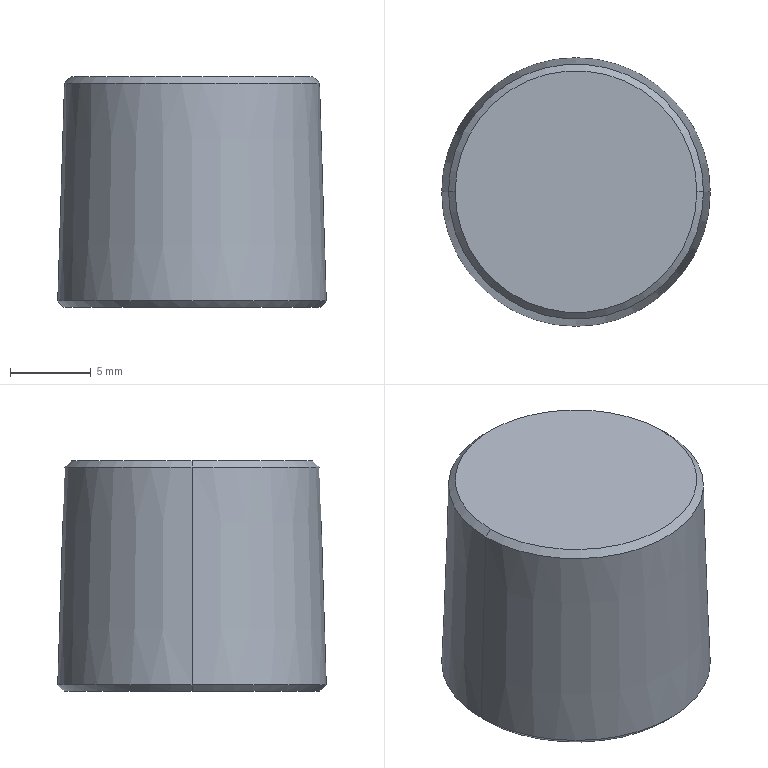Part | Creo | 1 solid | 15 faces | box 16.637 x 16.637 x 14.3 mm | volume 2739 mm3 | plane 9 | cone 6
STEP:
#1=CARTESIAN_POINT('',(-31.754,182.,-30.7));
#2=VERTEX_POINT('',#1);
#3=CARTESIAN_POINT('',(-46.729,182.,-30.7));
#4=VERTEX_POINT('',#3);
#5=CARTESIAN_POINT('',(-39.242,182.,-30.7));
#6=DIRECTION('',(0.,0.,1.));
#7=DIRECTION('',(1.,0.,0.));
#8=AXIS2_PLACEMENT_3D('',#5,#6,#7);
#9=CIRCLE('',#8,7.488);
#10=EDGE_CURVE('',#2,#4,#9,.T.);
#11=ORIENTED_EDGE('',*,*,#10,.F.);
#12=CARTESIAN_POINT('',(-39.242,182.,-30.7));
#13=DIRECTION('',(0.,0.,1.));
#14=DIRECTION('',(-1.,0.,0.));
#15=AXIS2_PLACEMENT_3D('',#12,#13,#14);
#16=CIRCLE('',#15,7.488);
#17=EDGE_CURVE('',#4,#2,#16,.T.);
#18=ORIENTED_EDGE('',*,*,#17,.F.);
#19=EDGE_LOOP('',(#11,#18));
#20=FACE_OUTER_BOUND('',#19,.F.);
#21=CARTESIAN_POINT('',(-47.129,182.,-30.7));
#22=DIRECTION('',(0.,0.,1.));
#23=DIRECTION('',(1.,0.,0.));
#24=AXIS2_PLACEMENT_3D('',#21,#22,#23);
#25=PLANE('',#24);
#26=ADVANCED_FACE('',(#20),#25,.T.);
#27=ORIENTED_EDGE('',*,*,#10,.T.);
#28=CARTESIAN_POINT('',(-47.142,182.,-31.1));
#29=VERTEX_POINT('',#28);
#30=CARTESIAN_POINT('',(-46.729,182.,-30.7));
#31=DIRECTION('',(-0.718,0.,-0.6961));
#32=VECTOR('',#31,0.5744);
#33=LINE('',#30,#32);
#34=EDGE_CURVE('',#4,#29,#33,.T.);
#35=ORIENTED_EDGE('',*,*,#34,.T.);
#36=CARTESIAN_POINT('',(-31.341,182.,-31.1));
#37=VERTEX_POINT('',#36);
#38=CARTESIAN_POINT('',(-39.242,182.,-31.1));
#39=DIRECTION('',(0.,0.,1.));
#40=DIRECTION('',(1.,0.,0.));
#41=AXIS2_PLACEMENT_3D('',#38,#39,#40);
#42=CIRCLE('',#41,7.9);
#43=EDGE_CURVE('',#37,#29,#42,.T.);
#44=ORIENTED_EDGE('',*,*,#43,.F.);
#45=CARTESIAN_POINT('',(-31.754,182.,-30.7));
#46=DIRECTION('',(0.718,0.,-0.6961));
#47=VECTOR('',#46,0.5744);
#48=LINE('',#45,#47);
#49=EDGE_CURVE('',#2,#37,#48,.T.);
#50=ORIENTED_EDGE('',*,*,#49,.F.);
#51=EDGE_LOOP('',(#27,#35,#44,#50));
#52=FACE_OUTER_BOUND('',#51,.F.);
#53=CARTESIAN_POINT('',(-39.242,182.,-30.9));
#54=DIRECTION('',(0.,0.,-1.));
#55=DIRECTION('',(-1.,0.,0.));
#56=AXIS2_PLACEMENT_3D('',#53,#54,#55);
#57=CONICAL_SURFACE('',#56,7.694,45.888);
#58=ADVANCED_FACE('',(#52),#57,.T.);
#59=ORIENTED_EDGE('',*,*,#17,.T.);
#60=ORIENTED_EDGE('',*,*,#49,.T.);
#61=CARTESIAN_POINT('',(-39.242,182.,-31.1));
#62=DIRECTION('',(0.,0.,1.));
#63=DIRECTION('',(-1.,0.,0.));
#64=AXIS2_PLACEMENT_3D('',#61,#62,#63);
#65=CIRCLE('',#64,7.9);
#66=EDGE_CURVE('',#29,#37,#65,.T.);
#67=ORIENTED_EDGE('',*,*,#66,.F.);
#68=ORIENTED_EDGE('',*,*,#34,.F.);
#69=EDGE_LOOP('',(#59,#60,#67,#68));
#70=FACE_OUTER_BOUND('',#69,.F.);
#71=CARTESIAN_POINT('',(-39.242,182.,-30.9));
#72=DIRECTION('',(0.,0.,-1.));
#73=DIRECTION('',(-1.,0.,0.));
#74=AXIS2_PLACEMENT_3D('',#71,#72,#73);
#75=CONICAL_SURFACE('',#74,7.694,45.888);
#76=ADVANCED_FACE('',(#70),#75,.T.);
#77=ORIENTED_EDGE('',*,*,#66,.T.);
#78=CARTESIAN_POINT('',(-30.923,182.,-44.6));
#79=VERTEX_POINT('',#78);
#80=CARTESIAN_POINT('',(-31.341,182.,-31.1));
#81=DIRECTION('',(0.03097,0.,-0.9995));
#82=VECTOR('',#81,13.507);
#83=LINE('',#80,#82);
#84=EDGE_CURVE('',#37,#79,#83,.T.);
#85=ORIENTED_EDGE('',*,*,#84,.T.);
#86=CARTESIAN_POINT('',(-47.56,182.,-44.6));
#87=VERTEX_POINT('',#86);
#88=CARTESIAN_POINT('',(-39.242,182.,-44.6));
#89=DIRECTION('',(0.,0.,-1.));
#90=DIRECTION('',(1.,0.,0.));
#91=AXIS2_PLACEMENT_3D('',#88,#89,#90);
#92=CIRCLE('',#91,8.319);
#93=EDGE_CURVE('',#79,#87,#92,.T.);
#94=ORIENTED_EDGE('',*,*,#93,.T.);
#95=CARTESIAN_POINT('',(-47.142,182.,-31.1));
#96=DIRECTION('',(-0.03097,0.,-0.9995));
#97=VECTOR('',#96,13.507);
#98=LINE('',#95,#97);
#99=EDGE_CURVE('',#29,#87,#98,.T.);
#100=ORIENTED_EDGE('',*,*,#99,.F.);
#101=EDGE_LOOP('',(#77,#85,#94,#100));
#102=FACE_OUTER_BOUND('',#101,.F.);
#103=CARTESIAN_POINT('',(-39.242,182.,-37.85));
#104=DIRECTION('',(0.,0.,-1.));
#105=DIRECTION('',(-1.,0.,0.));
#106=AXIS2_PLACEMENT_3D('',#103,#104,#105);
#107=CONICAL_SURFACE('',#106,8.109,1.775);
#108=ADVANCED_FACE('',(#102),#107,.T.);
#109=ORIENTED_EDGE('',*,*,#43,.T.);
#110=ORIENTED_EDGE('',*,*,#99,.T.);
#111=CARTESIAN_POINT('',(-39.242,182.,-44.6));
#112=DIRECTION('',(0.,0.,-1.));
#113=DIRECTION('',(-1.,0.,0.));
#114=AXIS2_PLACEMENT_3D('',#111,#112,#113);
#115=CIRCLE('',#114,8.319);
#116=EDGE_CURVE('',#87,#79,#115,.T.);
#117=ORIENTED_EDGE('',*,*,#116,.T.);
#118=ORIENTED_EDGE('',*,*,#84,.F.);
#119=EDGE_LOOP('',(#109,#110,#117,#118));
#120=FACE_OUTER_BOUND('',#119,.F.);
#121=CARTESIAN_POINT('',(-39.242,182.,-37.85));
#122=DIRECTION('',(0.,0.,-1.));
#123=DIRECTION('',(-1.,0.,0.));
#124=AXIS2_PLACEMENT_3D('',#121,#122,#123);
#125=CONICAL_SURFACE('',#124,8.109,1.775);
#126=ADVANCED_FACE('',(#120),#125,.T.);
#127=ORIENTED_EDGE('',*,*,#116,.F.);
#128=CARTESIAN_POINT('',(-47.173,182.,-45.));
#129=VERTEX_POINT('',#128);
#130=CARTESIAN_POINT('',(-47.173,182.,-45.));
#131=DIRECTION('',(-0.6961,0.,0.718));
#132=VECTOR('',#131,0.5569);
#133=LINE('',#130,#132);
#134=EDGE_CURVE('',#129,#87,#133,.T.);
#135=ORIENTED_EDGE('',*,*,#134,.F.);
#136=CARTESIAN_POINT('',(-31.311,182.,-45.));
#137=VERTEX_POINT('',#136);
#138=CARTESIAN_POINT('',(-39.242,182.,-45.));
#139=DIRECTION('',(0.,0.,-1.));
#140=DIRECTION('',(-1.,0.,0.));
#141=AXIS2_PLACEMENT_3D('',#138,#139,#140);
#142=CIRCLE('',#141,7.931);
#143=EDGE_CURVE('',#129,#137,#142,.T.);
#144=ORIENTED_EDGE('',*,*,#143,.T.);
#145=CARTESIAN_POINT('',(-31.311,182.,-45.));
#146=DIRECTION('',(0.6961,0.,0.718));
#147=VECTOR('',#146,0.5569);
#148=LINE('',#145,#147);
#149=EDGE_CURVE('',#137,#79,#148,.T.);
#150=ORIENTED_EDGE('',*,*,#149,.T.);
#151=EDGE_LOOP('',(#127,#135,#144,#150));
#152=FACE_OUTER_BOUND('',#151,.F.);
#153=CARTESIAN_POINT('',(-39.242,182.,-44.8));
#154=DIRECTION('',(0.,0.,1.));
#155=DIRECTION('',(1.,0.,0.));
#156=AXIS2_PLACEMENT_3D('',#153,#154,#155);
#157=CONICAL_SURFACE('',#156,8.125,44.112);
#158=ADVANCED_FACE('',(#152),#157,.T.);
#159=ORIENTED_EDGE('',*,*,#93,.F.);
#160=ORIENTED_EDGE('',*,*,#149,.F.);
#161=CARTESIAN_POINT('',(-39.242,182.,-45.));
#162=DIRECTION('',(0.,0.,-1.));
#163=DIRECTION('',(1.,0.,0.));
#164=AXIS2_PLACEMENT_3D('',#161,#162,#163);
#165=CIRCLE('',#164,7.931);
#166=EDGE_CURVE('',#137,#129,#165,.T.);
#167=ORIENTED_EDGE('',*,*,#166,.T.);
#168=ORIENTED_EDGE('',*,*,#134,.T.);
#169=EDGE_LOOP('',(#159,#160,#167,#168));
#170=FACE_OUTER_BOUND('',#169,.F.);
#171=CARTESIAN_POINT('',(-39.242,182.,-44.8));
#172=DIRECTION('',(0.,0.,1.));
#173=DIRECTION('',(1.,0.,0.));
#174=AXIS2_PLACEMENT_3D('',#171,#172,#173);
#175=CONICAL_SURFACE('',#174,8.125,44.112);
#176=ADVANCED_FACE('',(#170),#175,.T.);
#177=ORIENTED_EDGE('',*,*,#143,.F.);
#178=ORIENTED_EDGE('',*,*,#166,.F.);
#179=EDGE_LOOP('',(#177,#178));
#180=FACE_OUTER_BOUND('',#179,.F.);
#181=CARTESIAN_POINT('',(-37.242,178.536,-45.));
#182=VERTEX_POINT('',#181);
#183=CARTESIAN_POINT('',(-35.242,182.,-45.));
#184=VERTEX_POINT('',#183);
#185=CARTESIAN_POINT('',(-37.242,178.536,-45.));
#186=DIRECTION('',(0.5,0.866,0.));
#187=VECTOR('',#186,4.);
#188=LINE('',#185,#187);
#189=EDGE_CURVE('',#182,#184,#188,.T.);
#190=ORIENTED_EDGE('',*,*,#189,.F.);
#191=CARTESIAN_POINT('',(-41.242,178.536,-45.));
#192=VERTEX_POINT('',#191);
#193=CARTESIAN_POINT('',(-41.242,178.536,-45.));
#194=DIRECTION('',(1.,0.,0.));
#195=VECTOR('',#194,4.);
#196=LINE('',#193,#195);
#197=EDGE_CURVE('',#192,#182,#196,.T.);
#198=ORIENTED_EDGE('',*,*,#197,.F.);
#199=CARTESIAN_POINT('',(-43.242,182.,-45.));
#200=VERTEX_POINT('',#199);
#201=CARTESIAN_POINT('',(-43.242,182.,-45.));
#202=DIRECTION('',(0.5,-0.866,0.));
#203=VECTOR('',#202,4.);
#204=LINE('',#201,#203);
#205=EDGE_CURVE('',#200,#192,#204,.T.);
#206=ORIENTED_EDGE('',*,*,#205,.F.);
#207=CARTESIAN_POINT('',(-41.242,185.464,-45.));
#208=VERTEX_POINT('',#207);
#209=CARTESIAN_POINT('',(-41.242,185.464,-45.));
#210=DIRECTION('',(-0.5,-0.866,0.));
#211=VECTOR('',#210,4.);
#212=LINE('',#209,#211);
#213=EDGE_CURVE('',#208,#200,#212,.T.);
#214=ORIENTED_EDGE('',*,*,#213,.F.);
#215=CARTESIAN_POINT('',(-37.242,185.464,-45.));
#216=VERTEX_POINT('',#215);
#217=CARTESIAN_POINT('',(-37.242,185.464,-45.));
#218=DIRECTION('',(-1.,0.,0.));
#219=VECTOR('',#218,4.);
#220=LINE('',#217,#219);
#221=EDGE_CURVE('',#216,#208,#220,.T.);
#222=ORIENTED_EDGE('',*,*,#221,.F.);
#223=CARTESIAN_POINT('',(-35.242,182.,-45.));
#224=DIRECTION('',(-0.5,0.866,0.));
#225=VECTOR('',#224,4.);
#226=LINE('',#223,#225);
#227=EDGE_CURVE('',#184,#216,#226,.T.);
#228=ORIENTED_EDGE('',*,*,#227,.F.);
#229=EDGE_LOOP('',(#190,#198,#206,#214,#222,#228));
#230=FACE_BOUND('',#229,.F.);
#231=CARTESIAN_POINT('',(-39.242,182.,-45.));
#232=DIRECTION('',(0.,0.,-1.));
#233=DIRECTION('',(-1.,0.,0.));
#234=AXIS2_PLACEMENT_3D('',#231,#232,#233);
#235=PLANE('',#234);
#236=ADVANCED_FACE('',(#180,#230),#235,.T.);
#237=ORIENTED_EDGE('',*,*,#189,.T.);
#238=CARTESIAN_POINT('',(-35.242,182.,-40.));
#239=VERTEX_POINT('',#238);
#240=CARTESIAN_POINT('',(-35.242,182.,-40.));
#241=DIRECTION('',(0.,0.,-1.));
#242=VECTOR('',#241,5.);
#243=LINE('',#240,#242);
#244=EDGE_CURVE('',#239,#184,#243,.T.);
#245=ORIENTED_EDGE('',*,*,#244,.F.);
#246=CARTESIAN_POINT('',(-37.242,178.536,-40.));
#247=VERTEX_POINT('',#246);
#248=CARTESIAN_POINT('',(-35.242,182.,-40.));
#249=DIRECTION('',(-0.5,-0.866,0.));
#250=VECTOR('',#249,4.);
#251=LINE('',#248,#250);
#252=EDGE_CURVE('',#239,#247,#251,.T.);
#253=ORIENTED_EDGE('',*,*,#252,.T.);
#254=CARTESIAN_POINT('',(-37.242,178.536,-40.));
#255=DIRECTION('',(0.,0.,-1.));
#256=VECTOR('',#255,5.);
#257=LINE('',#254,#256);
#258=EDGE_CURVE('',#247,#182,#257,.T.);
#259=ORIENTED_EDGE('',*,*,#258,.T.);
#260=EDGE_LOOP('',(#237,#245,#253,#259));
#261=FACE_OUTER_BOUND('',#260,.F.);
#262=CARTESIAN_POINT('',(-35.242,182.,-40.));
#263=DIRECTION('',(0.866,-0.5,0.));
#264=DIRECTION('',(-0.5,-0.866,0.));
#265=AXIS2_PLACEMENT_3D('',#262,#263,#264);
#266=PLANE('',#265);
#267=ADVANCED_FACE('',(#261),#266,.F.);
#268=ORIENTED_EDGE('',*,*,#227,.T.);
#269=CARTESIAN_POINT('',(-37.242,185.464,-40.));
#270=VERTEX_POINT('',#269);
#271=CARTESIAN_POINT('',(-37.242,185.464,-40.));
#272=DIRECTION('',(0.,0.,-1.));
#273=VECTOR('',#272,5.);
#274=LINE('',#271,#273);
#275=EDGE_CURVE('',#270,#216,#274,.T.);
#276=ORIENTED_EDGE('',*,*,#275,.F.);
#277=CARTESIAN_POINT('',(-37.242,185.464,-40.));
#278=DIRECTION('',(0.5,-0.866,0.));
#279=VECTOR('',#278,4.);
#280=LINE('',#277,#279);
#281=EDGE_CURVE('',#270,#239,#280,.T.);
#282=ORIENTED_EDGE('',*,*,#281,.T.);
#283=ORIENTED_EDGE('',*,*,#244,.T.);
#284=EDGE_LOOP('',(#268,#276,#282,#283));
#285=FACE_OUTER_BOUND('',#284,.F.);
#286=CARTESIAN_POINT('',(-37.242,185.464,-40.));
#287=DIRECTION('',(0.866,0.5,0.));
#288=DIRECTION('',(0.5,-0.866,0.));
#289=AXIS2_PLACEMENT_3D('',#286,#287,#288);
#290=PLANE('',#289);
#291=ADVANCED_FACE('',(#285),#290,.F.);
#292=ORIENTED_EDGE('',*,*,#221,.T.);
#293=CARTESIAN_POINT('',(-41.242,185.464,-40.));
#294=VERTEX_POINT('',#293);
#295=CARTESIAN_POINT('',(-41.242,185.464,-40.));
#296=DIRECTION('',(0.,0.,-1.));
#297=VECTOR('',#296,5.);
#298=LINE('',#295,#297);
#299=EDGE_CURVE('',#294,#208,#298,.T.);
#300=ORIENTED_EDGE('',*,*,#299,.F.);
#301=CARTESIAN_POINT('',(-41.242,185.464,-40.));
#302=DIRECTION('',(1.,0.,0.));
#303=VECTOR('',#302,4.);
#304=LINE('',#301,#303);
#305=EDGE_CURVE('',#294,#270,#304,.T.);
#306=ORIENTED_EDGE('',*,*,#305,.T.);
#307=ORIENTED_EDGE('',*,*,#275,.T.);
#308=EDGE_LOOP('',(#292,#300,#306,#307));
#309=FACE_OUTER_BOUND('',#308,.F.);
#310=CARTESIAN_POINT('',(-41.242,185.464,-40.));
#311=DIRECTION('',(0.,1.,0.));
#312=DIRECTION('',(1.,0.,0.));
#313=AXIS2_PLACEMENT_3D('',#310,#311,#312);
#314=PLANE('',#313);
#315=ADVANCED_FACE('',(#309),#314,.F.);
#316=ORIENTED_EDGE('',*,*,#213,.T.);
#317=CARTESIAN_POINT('',(-43.242,182.,-40.));
#318=VERTEX_POINT('',#317);
#319=CARTESIAN_POINT('',(-43.242,182.,-40.));
#320=DIRECTION('',(0.,0.,-1.));
#321=VECTOR('',#320,5.);
#322=LINE('',#319,#321);
#323=EDGE_CURVE('',#318,#200,#322,.T.);
#324=ORIENTED_EDGE('',*,*,#323,.F.);
#325=CARTESIAN_POINT('',(-43.242,182.,-40.));
#326=DIRECTION('',(0.5,0.866,0.));
#327=VECTOR('',#326,4.);
#328=LINE('',#325,#327);
#329=EDGE_CURVE('',#318,#294,#328,.T.);
#330=ORIENTED_EDGE('',*,*,#329,.T.);
#331=ORIENTED_EDGE('',*,*,#299,.T.);
#332=EDGE_LOOP('',(#316,#324,#330,#331));
#333=FACE_OUTER_BOUND('',#332,.F.);
#334=CARTESIAN_POINT('',(-43.242,182.,-40.));
#335=DIRECTION('',(-0.866,0.5,0.));
#336=DIRECTION('',(0.5,0.866,0.));
#337=AXIS2_PLACEMENT_3D('',#334,#335,#336);
#338=PLANE('',#337);
#339=ADVANCED_FACE('',(#333),#338,.F.);
#340=ORIENTED_EDGE('',*,*,#205,.T.);
#341=CARTESIAN_POINT('',(-41.242,178.536,-40.));
#342=VERTEX_POINT('',#341);
#343=CARTESIAN_POINT('',(-41.242,178.536,-40.));
#344=DIRECTION('',(0.,0.,-1.));
#345=VECTOR('',#344,5.);
#346=LINE('',#343,#345);
#347=EDGE_CURVE('',#342,#192,#346,.T.);
#348=ORIENTED_EDGE('',*,*,#347,.F.);
#349=CARTESIAN_POINT('',(-41.242,178.536,-40.));
#350=DIRECTION('',(-0.5,0.866,0.));
#351=VECTOR('',#350,4.);
#352=LINE('',#349,#351);
#353=EDGE_CURVE('',#342,#318,#352,.T.);
#354=ORIENTED_EDGE('',*,*,#353,.T.);
#355=ORIENTED_EDGE('',*,*,#323,.T.);
#356=EDGE_LOOP('',(#340,#348,#354,#355));
#357=FACE_OUTER_BOUND('',#356,.F.);
#358=CARTESIAN_POINT('',(-41.242,178.536,-40.));
#359=DIRECTION('',(-0.866,-0.5,0.));
#360=DIRECTION('',(-0.5,0.866,0.));
#361=AXIS2_PLACEMENT_3D('',#358,#359,#360);
#362=PLANE('',#361);
#363=ADVANCED_FACE('',(#357),#362,.F.);
#364=ORIENTED_EDGE('',*,*,#197,.T.);
#365=ORIENTED_EDGE('',*,*,#258,.F.);
#366=CARTESIAN_POINT('',(-37.242,178.536,-40.));
#367=DIRECTION('',(-1.,0.,0.));
#368=VECTOR('',#367,4.);
#369=LINE('',#366,#368);
#370=EDGE_CURVE('',#247,#342,#369,.T.);
#371=ORIENTED_EDGE('',*,*,#370,.T.);
#372=ORIENTED_EDGE('',*,*,#347,.T.);
#373=EDGE_LOOP('',(#364,#365,#371,#372));
#374=FACE_OUTER_BOUND('',#373,.F.);
#375=CARTESIAN_POINT('',(-37.242,178.536,-40.));
#376=DIRECTION('',(0.,-1.,0.));
#377=DIRECTION('',(-1.,0.,0.));
#378=AXIS2_PLACEMENT_3D('',#375,#376,#377);
#379=PLANE('',#378);
#380=ADVANCED_FACE('',(#374),#379,.F.);
#381=ORIENTED_EDGE('',*,*,#252,.F.);
#382=ORIENTED_EDGE('',*,*,#281,.F.);
#383=ORIENTED_EDGE('',*,*,#305,.F.);
#384=ORIENTED_EDGE('',*,*,#329,.F.);
#385=ORIENTED_EDGE('',*,*,#353,.F.);
#386=ORIENTED_EDGE('',*,*,#370,.F.);
#387=EDGE_LOOP('',(#381,#382,#383,#384,#385,#386));
#388=FACE_OUTER_BOUND('',#387,.F.);
#389=CARTESIAN_POINT('',(-39.242,182.,-40.));
#390=DIRECTION('',(0.,0.,-1.));
#391=DIRECTION('',(-1.,0.,0.));
#392=AXIS2_PLACEMENT_3D('',#389,#390,#391);
#393=PLANE('',#392);
#394=ADVANCED_FACE('',(#388),#393,.T.);
#395=CLOSED_SHELL('',(#26,#58,#76,#108,#126,#158,#176,#236,#267,#291,#315,#339,#363,#380,#394));
#396=MANIFOLD_SOLID_BREP('',#395);
#397=(LENGTH_UNIT()NAMED_UNIT(*)SI_UNIT(.MILLI.,.METRE.));
#398=UNCERTAINTY_MEASURE_WITH_UNIT(LENGTH_MEASURE(0.002753),#397,'','');
#399=(NAMED_UNIT(*)PLANE_ANGLE_UNIT()SI_UNIT($,.RADIAN.));
#400=PLANE_ANGLE_MEASURE_WITH_UNIT(PLANE_ANGLE_MEASURE(0.01745),#399);
#401=(CONVERSION_BASED_UNIT('DEGREE',#400)NAMED_UNIT(*)PLANE_ANGLE_UNIT());
#402=(NAMED_UNIT(*)SI_UNIT($,.STERADIAN.)SOLID_ANGLE_UNIT());
#403=(GEOMETRIC_REPRESENTATION_CONTEXT(3)GLOBAL_UNCERTAINTY_ASSIGNED_CONTEXT((#398))GLOBAL_UNIT_ASSIGNED_CONTEXT((#397,#401,#402))REPRESENTATION_CONTEXT('',''));
#404=ADVANCED_BREP_SHAPE_REPRESENTATION('',(#396),#403);